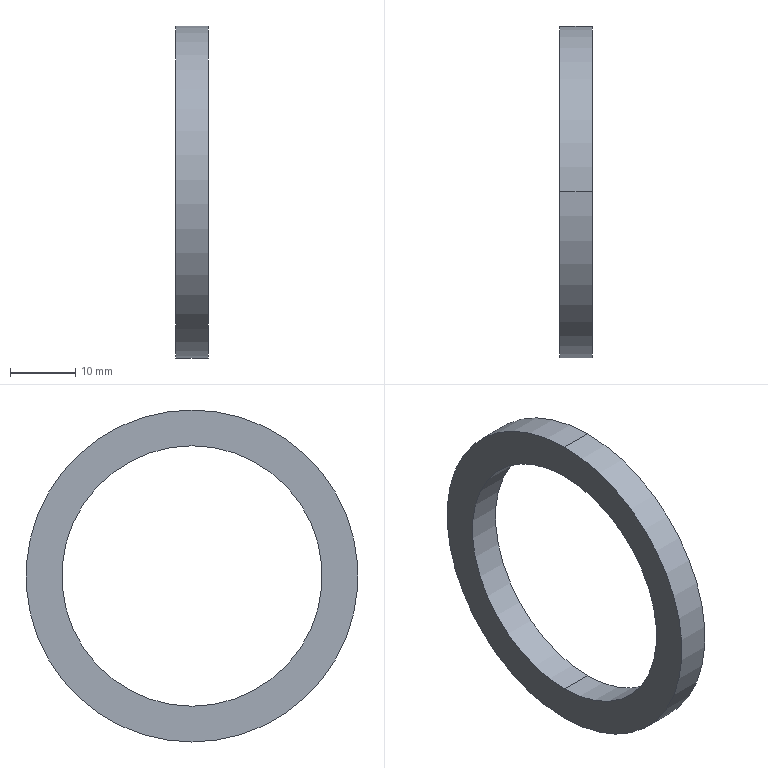Part | SolidWorks | features Revolution 1 | 1 solid | 6 faces | box 5 x 51 x 51 mm | volume 3931 mm3 | cylinder 4 | plane 2 | commonest cylinder face diameters 40 x2 51 x2
STEP:
#1=CARTESIAN_POINT('',(5.,0.,-20.));
#2=VERTEX_POINT('',#1);
#3=CARTESIAN_POINT('',(5.,0.,20.));
#4=VERTEX_POINT('',#3);
#5=CARTESIAN_POINT('',(5.,0.,0.));
#6=DIRECTION('',(-1.,0.,0.));
#7=DIRECTION('',(0.,0.,1.));
#8=AXIS2_PLACEMENT_3D('',#5,#6,#7);
#9=CIRCLE('',#8,20.);
#10=EDGE_CURVE('',#2,#4,#9,.T.);
#11=ORIENTED_EDGE('',*,*,#10,.F.);
#12=CARTESIAN_POINT('',(0.,0.,-20.));
#13=VERTEX_POINT('',#12);
#14=CARTESIAN_POINT('',(-329.824,0.,-20.));
#15=DIRECTION('',(-1.,0.,0.));
#16=VECTOR('',#15,1000.);
#17=LINE('',#14,#16);
#18=EDGE_CURVE('',#2,#13,#17,.T.);
#19=ORIENTED_EDGE('',*,*,#18,.T.);
#20=CARTESIAN_POINT('',(0.,0.,20.));
#21=VERTEX_POINT('',#20);
#22=CARTESIAN_POINT('',(0.,0.,0.));
#23=DIRECTION('',(-1.,0.,0.));
#24=DIRECTION('',(0.,0.,1.));
#25=AXIS2_PLACEMENT_3D('',#22,#23,#24);
#26=CIRCLE('',#25,20.);
#27=EDGE_CURVE('',#13,#21,#26,.T.);
#28=ORIENTED_EDGE('',*,*,#27,.T.);
#29=CARTESIAN_POINT('',(-329.824,0.,20.));
#30=DIRECTION('',(-1.,0.,0.));
#31=VECTOR('',#30,1000.);
#32=LINE('',#29,#31);
#33=EDGE_CURVE('',#4,#21,#32,.T.);
#34=ORIENTED_EDGE('',*,*,#33,.F.);
#35=EDGE_LOOP('',(#11,#19,#28,#34));
#36=FACE_OUTER_BOUND('',#35,.T.);
#37=CARTESIAN_POINT('',(-329.824,0.,0.));
#38=DIRECTION('',(-1.,0.,0.));
#39=DIRECTION('',(0.,0.,1.));
#40=AXIS2_PLACEMENT_3D('',#37,#38,#39);
#41=CYLINDRICAL_SURFACE('',#40,20.);
#42=ADVANCED_FACE('',(#36),#41,.F.);
#43=CARTESIAN_POINT('',(5.,0.,25.5));
#44=VERTEX_POINT('',#43);
#45=CARTESIAN_POINT('',(5.,0.,-25.5));
#46=VERTEX_POINT('',#45);
#47=CARTESIAN_POINT('',(5.,0.,0.));
#48=DIRECTION('',(-1.,0.,0.));
#49=DIRECTION('',(0.,0.,1.));
#50=AXIS2_PLACEMENT_3D('',#47,#48,#49);
#51=CIRCLE('',#50,25.5);
#52=EDGE_CURVE('',#44,#46,#51,.T.);
#53=ORIENTED_EDGE('',*,*,#52,.T.);
#54=CARTESIAN_POINT('',(0.,0.,-25.5));
#55=VERTEX_POINT('',#54);
#56=CARTESIAN_POINT('',(-329.824,0.,-25.5));
#57=DIRECTION('',(-1.,0.,0.));
#58=VECTOR('',#57,1000.);
#59=LINE('',#56,#58);
#60=EDGE_CURVE('',#46,#55,#59,.T.);
#61=ORIENTED_EDGE('',*,*,#60,.T.);
#62=CARTESIAN_POINT('',(0.,0.,25.5));
#63=VERTEX_POINT('',#62);
#64=CARTESIAN_POINT('',(0.,0.,0.));
#65=DIRECTION('',(-1.,0.,0.));
#66=DIRECTION('',(0.,0.,1.));
#67=AXIS2_PLACEMENT_3D('',#64,#65,#66);
#68=CIRCLE('',#67,25.5);
#69=EDGE_CURVE('',#63,#55,#68,.T.);
#70=ORIENTED_EDGE('',*,*,#69,.F.);
#71=CARTESIAN_POINT('',(-329.824,0.,25.5));
#72=DIRECTION('',(-1.,0.,0.));
#73=VECTOR('',#72,1000.);
#74=LINE('',#71,#73);
#75=EDGE_CURVE('',#44,#63,#74,.T.);
#76=ORIENTED_EDGE('',*,*,#75,.F.);
#77=EDGE_LOOP('',(#53,#61,#70,#76));
#78=FACE_OUTER_BOUND('',#77,.T.);
#79=CARTESIAN_POINT('',(-329.824,0.,0.));
#80=DIRECTION('',(-1.,0.,0.));
#81=DIRECTION('',(0.,0.,1.));
#82=AXIS2_PLACEMENT_3D('',#79,#80,#81);
#83=CYLINDRICAL_SURFACE('',#82,25.5);
#84=ADVANCED_FACE('',(#78),#83,.T.);
#85=CARTESIAN_POINT('',(0.,0.,0.));
#86=DIRECTION('',(-1.,0.,0.));
#87=DIRECTION('',(0.,0.,1.));
#88=AXIS2_PLACEMENT_3D('',#85,#86,#87);
#89=CIRCLE('',#88,20.);
#90=EDGE_CURVE('',#21,#13,#89,.T.);
#91=ORIENTED_EDGE('',*,*,#90,.F.);
#92=ORIENTED_EDGE('',*,*,#27,.F.);
#93=EDGE_LOOP('',(#91,#92));
#94=FACE_BOUND('',#93,.T.);
#95=ORIENTED_EDGE('',*,*,#69,.T.);
#96=CARTESIAN_POINT('',(0.,0.,0.));
#97=DIRECTION('',(-1.,0.,0.));
#98=DIRECTION('',(0.,0.,1.));
#99=AXIS2_PLACEMENT_3D('',#96,#97,#98);
#100=CIRCLE('',#99,25.5);
#101=EDGE_CURVE('',#55,#63,#100,.T.);
#102=ORIENTED_EDGE('',*,*,#101,.T.);
#103=EDGE_LOOP('',(#95,#102));
#104=FACE_OUTER_BOUND('',#103,.T.);
#105=CARTESIAN_POINT('',(0.,0.,-20.));
#106=DIRECTION('',(1.,0.,0.));
#107=DIRECTION('',(0.,0.,-1.));
#108=AXIS2_PLACEMENT_3D('',#105,#106,#107);
#109=PLANE('',#108);
#110=ADVANCED_FACE('',(#94,#104),#109,.F.);
#111=ORIENTED_EDGE('',*,*,#60,.F.);
#112=CARTESIAN_POINT('',(5.,0.,0.));
#113=DIRECTION('',(-1.,0.,0.));
#114=DIRECTION('',(0.,0.,1.));
#115=AXIS2_PLACEMENT_3D('',#112,#113,#114);
#116=CIRCLE('',#115,25.5);
#117=EDGE_CURVE('',#46,#44,#116,.T.);
#118=ORIENTED_EDGE('',*,*,#117,.T.);
#119=ORIENTED_EDGE('',*,*,#75,.T.);
#120=ORIENTED_EDGE('',*,*,#101,.F.);
#121=EDGE_LOOP('',(#111,#118,#119,#120));
#122=FACE_OUTER_BOUND('',#121,.T.);
#123=CARTESIAN_POINT('',(-329.824,0.,0.));
#124=DIRECTION('',(-1.,0.,0.));
#125=DIRECTION('',(0.,0.,1.));
#126=AXIS2_PLACEMENT_3D('',#123,#124,#125);
#127=CYLINDRICAL_SURFACE('',#126,25.5);
#128=ADVANCED_FACE('',(#122),#127,.T.);
#129=ORIENTED_EDGE('',*,*,#52,.F.);
#130=ORIENTED_EDGE('',*,*,#117,.F.);
#131=EDGE_LOOP('',(#129,#130));
#132=FACE_OUTER_BOUND('',#131,.T.);
#133=CARTESIAN_POINT('',(5.,0.,0.));
#134=DIRECTION('',(-1.,0.,0.));
#135=DIRECTION('',(0.,0.,1.));
#136=AXIS2_PLACEMENT_3D('',#133,#134,#135);
#137=CIRCLE('',#136,20.);
#138=EDGE_CURVE('',#4,#2,#137,.T.);
#139=ORIENTED_EDGE('',*,*,#138,.T.);
#140=ORIENTED_EDGE('',*,*,#10,.T.);
#141=EDGE_LOOP('',(#139,#140));
#142=FACE_BOUND('',#141,.T.);
#143=CARTESIAN_POINT('',(5.,0.,-20.));
#144=DIRECTION('',(-1.,0.,0.));
#145=DIRECTION('',(0.,0.,1.));
#146=AXIS2_PLACEMENT_3D('',#143,#144,#145);
#147=PLANE('',#146);
#148=ADVANCED_FACE('',(#132,#142),#147,.F.);
#149=ORIENTED_EDGE('',*,*,#18,.F.);
#150=ORIENTED_EDGE('',*,*,#138,.F.);
#151=ORIENTED_EDGE('',*,*,#33,.T.);
#152=ORIENTED_EDGE('',*,*,#90,.T.);
#153=EDGE_LOOP('',(#149,#150,#151,#152));
#154=FACE_OUTER_BOUND('',#153,.T.);
#155=CARTESIAN_POINT('',(-329.824,0.,0.));
#156=DIRECTION('',(-1.,0.,0.));
#157=DIRECTION('',(0.,0.,1.));
#158=AXIS2_PLACEMENT_3D('',#155,#156,#157);
#159=CYLINDRICAL_SURFACE('',#158,20.);
#160=ADVANCED_FACE('',(#154),#159,.F.);
#161=CLOSED_SHELL('',(#42,#84,#110,#128,#148,#160));
#162=MANIFOLD_SOLID_BREP('',#161);
#163=CARTESIAN_POINT('',(0.,0.,0.));
#164=DIRECTION('',(0.,0.,1.));
#165=DIRECTION('',(1.,0.,0.));
#166=AXIS2_PLACEMENT_3D('',#163,#164,#165);
#167=(LENGTH_UNIT()NAMED_UNIT(*)SI_UNIT(.MILLI.,.METRE.));
#168=UNCERTAINTY_MEASURE_WITH_UNIT(LENGTH_MEASURE(0.00001),#167,'','');
#169=(NAMED_UNIT(*)PLANE_ANGLE_UNIT()SI_UNIT($,.RADIAN.));
#170=(NAMED_UNIT(*)SI_UNIT($,.STERADIAN.)SOLID_ANGLE_UNIT());
#171=(GEOMETRIC_REPRESENTATION_CONTEXT(3)GLOBAL_UNCERTAINTY_ASSIGNED_CONTEXT((#168))GLOBAL_UNIT_ASSIGNED_CONTEXT((#167,#169,#170))REPRESENTATION_CONTEXT('',''));
#172=ADVANCED_BREP_SHAPE_REPRESENTATION('',(#162,#166),#171);